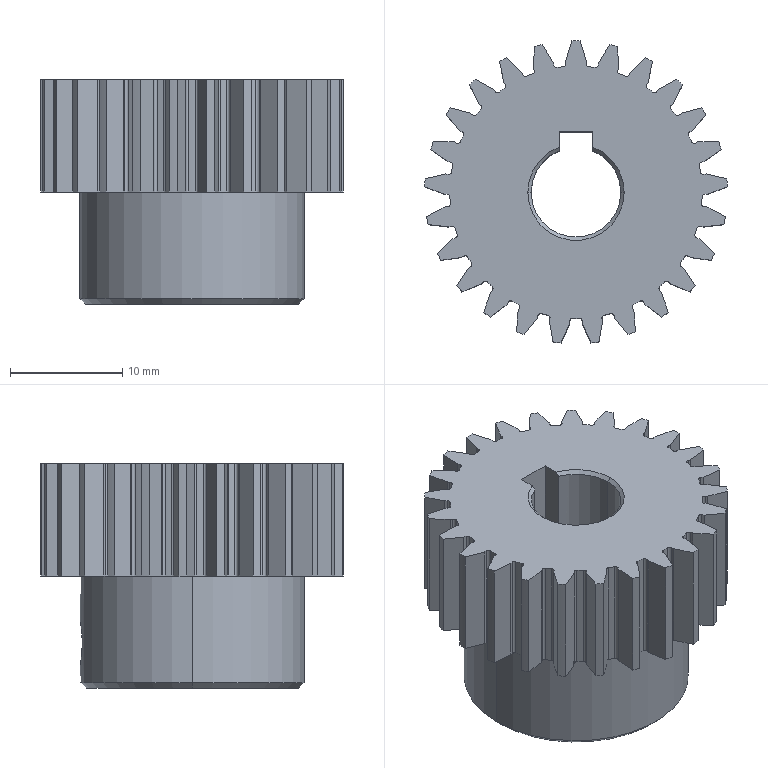Part | SolidWorks | features BaseBody 1 | 1 solid | 238 faces | box 26.982 x 26.934 x 20 mm | volume 6760 mm3 | cylinder 119 | plane 109 | cone 10 | commonest cylinder face diameters 0.5 x62 22.5 x25 27 x25 8 x3 3.242 x2 20 x2